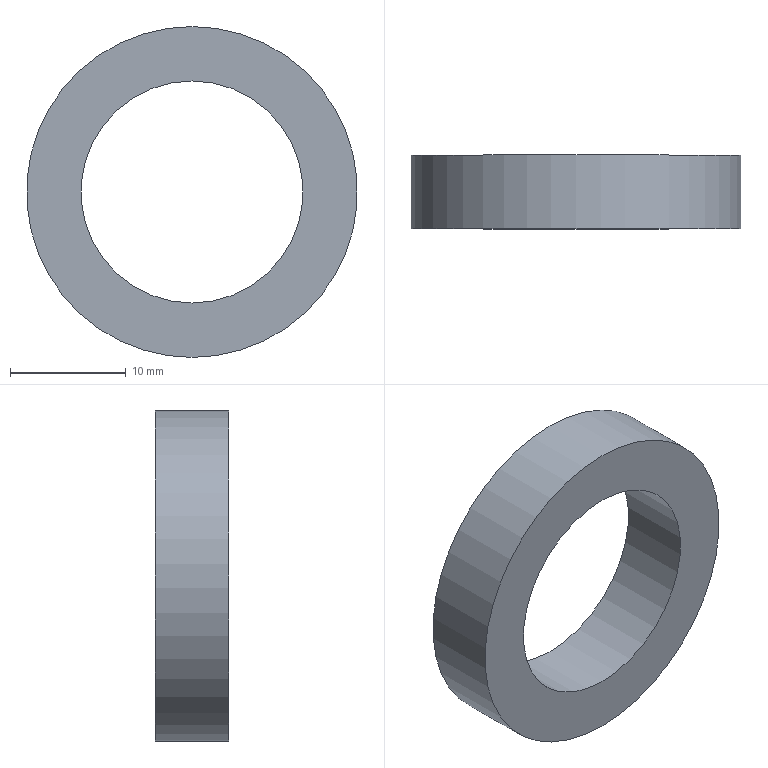Part | NX | features MG0330 trunion parts 24(trunion group) 2 | 1 solid | 4 faces | box 28.575 x 6.35 x 28.575 mm | volume 2238 mm3 | cylinder 2 | plane 2 | commonest cylinder face diameters 19.177 x1 28.575 x1
STEP:
#1=CARTESIAN_POINT('',(0.,-15.875,-9.588));
#2=VERTEX_POINT('',#1);
#3=CARTESIAN_POINT('',(0.,-15.875,0.));
#4=DIRECTION('',(0.,-1.,0.));
#5=DIRECTION('',(0.,0.,-1.));
#6=AXIS2_PLACEMENT_3D('',#3,#4,#5);
#7=CIRCLE('',#6,9.588);
#8=EDGE_CURVE('',#2,#2,#7,.T.);
#9=ORIENTED_EDGE('',*,*,#8,.T.);
#10=EDGE_LOOP('',(#9));
#11=FACE_BOUND('',#10,.T.);
#12=CARTESIAN_POINT('',(0.,-9.525,-9.588));
#13=VERTEX_POINT('',#12);
#14=CARTESIAN_POINT('',(0.,-9.525,0.));
#15=DIRECTION('',(0.,-1.,0.));
#16=DIRECTION('',(0.,0.,-1.));
#17=AXIS2_PLACEMENT_3D('',#14,#15,#16);
#18=CIRCLE('',#17,9.588);
#19=EDGE_CURVE('',#13,#13,#18,.T.);
#20=ORIENTED_EDGE('',*,*,#19,.F.);
#21=EDGE_LOOP('',(#20));
#22=FACE_BOUND('',#21,.T.);
#23=CARTESIAN_POINT('',(0.,0.,0.));
#24=DIRECTION('',(0.,-1.,0.));
#25=DIRECTION('',(0.,0.,-1.));
#26=AXIS2_PLACEMENT_3D('',#23,#24,#25);
#27=CYLINDRICAL_SURFACE('',#26,9.588);
#28=ADVANCED_FACE('',(#11,#22),#27,.F.);
#29=CARTESIAN_POINT('',(0.,-15.875,-14.287));
#30=VERTEX_POINT('',#29);
#31=CARTESIAN_POINT('',(0.,-15.875,0.));
#32=DIRECTION('',(0.,-1.,0.));
#33=DIRECTION('',(0.,0.,-1.));
#34=AXIS2_PLACEMENT_3D('',#31,#32,#33);
#35=CIRCLE('',#34,14.287);
#36=EDGE_CURVE('',#30,#30,#35,.T.);
#37=ORIENTED_EDGE('',*,*,#36,.T.);
#38=EDGE_LOOP('',(#37));
#39=FACE_BOUND('',#38,.T.);
#40=ORIENTED_EDGE('',*,*,#8,.F.);
#41=EDGE_LOOP('',(#40));
#42=FACE_BOUND('',#41,.T.);
#43=CARTESIAN_POINT('',(9.588,-15.875,0.));
#44=DIRECTION('',(0.,-1.,0.));
#45=DIRECTION('',(0.,0.,-1.));
#46=AXIS2_PLACEMENT_3D('',#43,#44,#45);
#47=PLANE('',#46);
#48=ADVANCED_FACE('',(#39,#42),#47,.T.);
#49=CARTESIAN_POINT('',(0.,-9.525,-14.287));
#50=VERTEX_POINT('',#49);
#51=CARTESIAN_POINT('',(0.,-9.525,0.));
#52=DIRECTION('',(0.,-1.,0.));
#53=DIRECTION('',(0.,0.,-1.));
#54=AXIS2_PLACEMENT_3D('',#51,#52,#53);
#55=CIRCLE('',#54,14.287);
#56=EDGE_CURVE('',#50,#50,#55,.T.);
#57=ORIENTED_EDGE('',*,*,#56,.T.);
#58=EDGE_LOOP('',(#57));
#59=FACE_BOUND('',#58,.T.);
#60=ORIENTED_EDGE('',*,*,#36,.F.);
#61=EDGE_LOOP('',(#60));
#62=FACE_BOUND('',#61,.T.);
#63=CARTESIAN_POINT('',(0.,0.,0.));
#64=DIRECTION('',(0.,-1.,0.));
#65=DIRECTION('',(0.,0.,-1.));
#66=AXIS2_PLACEMENT_3D('',#63,#64,#65);
#67=CYLINDRICAL_SURFACE('',#66,14.287);
#68=ADVANCED_FACE('',(#59,#62),#67,.T.);
#69=ORIENTED_EDGE('',*,*,#19,.T.);
#70=EDGE_LOOP('',(#69));
#71=FACE_BOUND('',#70,.T.);
#72=ORIENTED_EDGE('',*,*,#56,.F.);
#73=EDGE_LOOP('',(#72));
#74=FACE_BOUND('',#73,.T.);
#75=CARTESIAN_POINT('',(9.588,-9.525,0.));
#76=DIRECTION('',(0.,1.,0.));
#77=DIRECTION('',(0.,0.,1.));
#78=AXIS2_PLACEMENT_3D('',#75,#76,#77);
#79=PLANE('',#78);
#80=ADVANCED_FACE('',(#71,#74),#79,.T.);
#81=CLOSED_SHELL('',(#28,#48,#68,#80));
#82=MANIFOLD_SOLID_BREP('',#81);
#83=(LENGTH_UNIT()NAMED_UNIT(*)SI_UNIT(.MILLI.,.METRE.));
#84=UNCERTAINTY_MEASURE_WITH_UNIT(LENGTH_MEASURE(0.00001),#83,'','');
#85=(NAMED_UNIT(*)PLANE_ANGLE_UNIT()SI_UNIT($,.RADIAN.));
#86=(NAMED_UNIT(*)SI_UNIT($,.STERADIAN.)SOLID_ANGLE_UNIT());
#87=(GEOMETRIC_REPRESENTATION_CONTEXT(3)GLOBAL_UNCERTAINTY_ASSIGNED_CONTEXT((#84))GLOBAL_UNIT_ASSIGNED_CONTEXT((#83,#85,#86))REPRESENTATION_CONTEXT('',''));
#88=ADVANCED_BREP_SHAPE_REPRESENTATION('',(#82),#87);